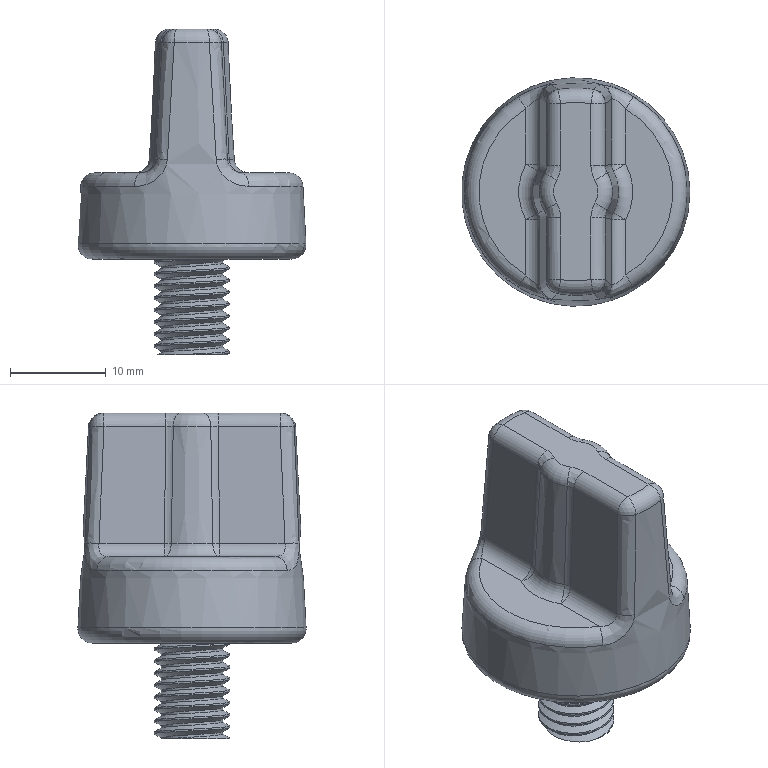Part | STEP file | Base_plate_001 | 1 solid | 57 faces | box 23.839 x 23.839 x 34 mm | volume 6540 mm3 | spline 18 | cylinder 10 | plane 9 | torus 9 | sphere 8 | cone 3 | commonest cylinder face diameters 3 x8 6.446 x1 7.866 x1